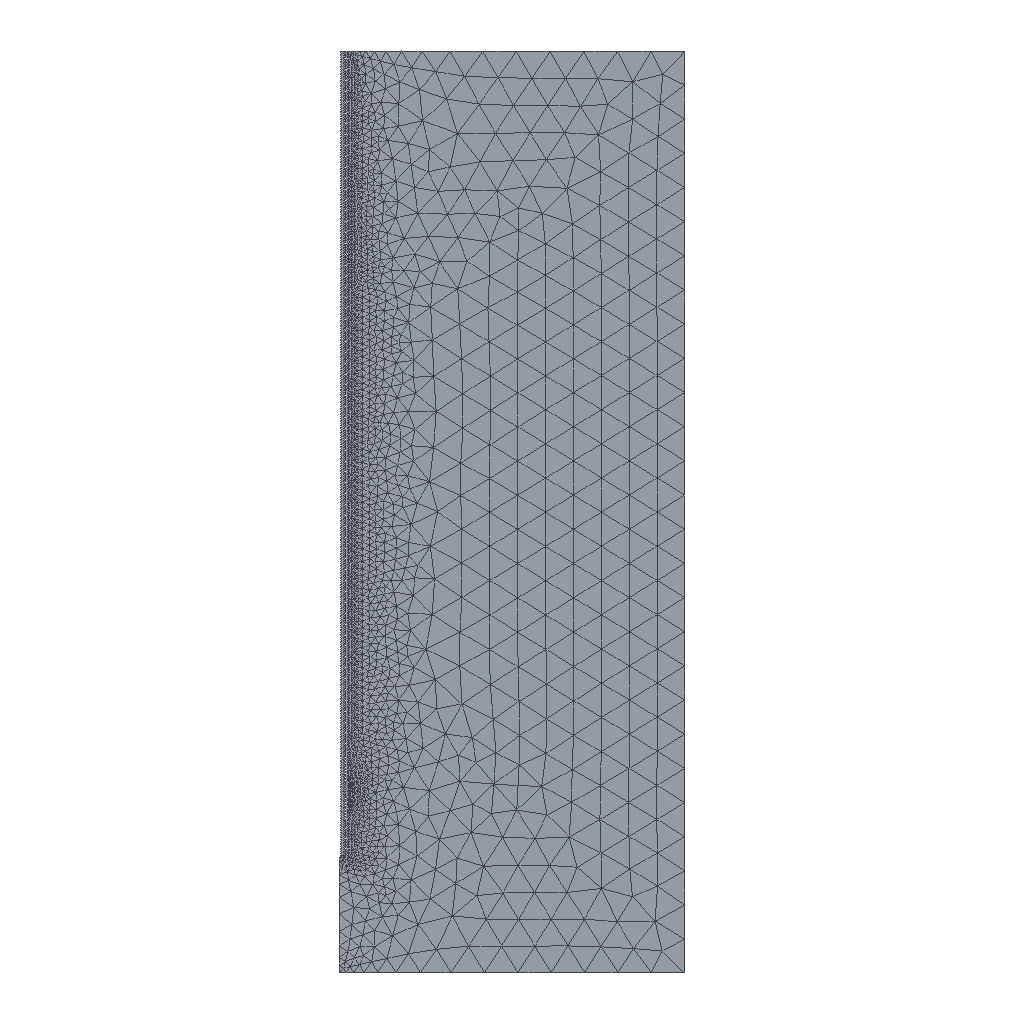Simulation study | comsol
Notes in the study folder:
k_liver 0.56[W/(m*K)] Thermal conductivity liver
rho_blood 1e3[kg/m^3] Density blood
Cp_blood 3639[J/(kg*K)] Heat capacity blood
omega_blood 3.6e-3[1/s] Blood perfusion rate
T_blood 37[degC] Temperature blood
P_in 10[W] Microwave power input
f 2.45[GHz] Microwave frequency
eps_diel 2.6[1] Dielectric relative permittivity
eps_cat 2.6[1] Catheter relative permittivity
eps_liver 43.03[1] Liver relative permittivity
sigma_liver 1.69[S/m] Conductivity liver
rho_liver 1038[kg/m^3] Liver density
Cp_liver 4187[J/(kg*K)] Liver heat capacity
sigma_cat 1e-6[S/m] Catheter conductivity
mur_cat 1[1] Catheter relative permeability
k_ptfe 0.25[W/(m*K)] Thermal conductivity PTFE
rho_ptfe 2200[kg/m^3] Density PTFE
Cp_ptfe 1300[J/(kg*K)] PTFE heat capacity
sigma_diel 1e-6[S/m] Microwave center feed
mur_diel 1[1] Relative permeability dielectric
mur_liver 1[1] Relative permeability liver
Set-up summary:
category,name,step,type,value,unit,region
solver,comsol,,COMSOL Multiphysics 6.4 (Build: 293)
units,SI; geometry length unit m,,stated,COMSOL default unit system (SI)
analysis,Study 1,,Frequency + Stationary,space_dimension=2D
load_step,std1/freq,std1/freq,Frequency + Stationary,type=Frequency; frequencies=f
load_step,std1/stat,std1/stat,Frequency + Stationary,type=Stationary
mesh,nodes,,,4184
mesh,elements,,,7113
element_type,tri,,,7113
element_type,edg,,,1524
element_type,vtx,,,18
component,mod1,,2D,geometry=geom1; domains=4
physics,Electromagnetic Waves (emw),mod1,ElectromagneticWaves,E(Er Ephi Ez)
physics,Heat Transfer (ht),mod1,BioHeat,"T(T), discontinuousdamagedtissueindicator(discontinuousdamagedtissueindicator), continuousdamagedtissueindicator(continuousdamagedtissueindicator), thermaldamageindicator(thermaldamageindicator), radiativeintensity(radiativeintensity), incidentradiation(incidentradiation), surfaceradiosity(surfaceradiosity)"
parameter,k_liver,,,0.56[W/(m*K)]
parameter,rho_blood,,,1e3[kg/m^3]
parameter,Cp_blood,,,3639[J/(kg*K)]
parameter,omega_blood,,,3.6e-3[1/s]
parameter,T_blood,,,37[degC]
parameter,P_in,,,10[W]
parameter,f,,,2.45[GHz]
parameter,eps_diel,,,2.6[1]
parameter,eps_cat,,,2.6[1]
parameter,eps_liver,,,43.03[1]
parameter,sigma_liver,,,1.69[S/m]
parameter,rho_liver,,,1038[kg/m^3]
parameter,Cp_liver,,,4187[J/(kg*K)]
parameter,sigma_cat,,,1e-6[S/m]
parameter,mur_cat,,,1[1]
parameter,k_ptfe,,,0.25[W/(m*K)]
parameter,rho_ptfe,,,2200[kg/m^3]
parameter,Cp_ptfe,,,1300[J/(kg*K)]
parameter,sigma_diel,,,1e-6[S/m]
parameter,mur_diel,,,1[1]
parameter,mur_liver,,,1[1]
material,Liver Tissue,,electricconductivity,sigma_liver,,selection [1]
material,Liver Tissue,,relpermittivity,eps_liver,,selection [1]
material,Liver Tissue,,relpermeability,mur_liver,,selection [1]
material,Liver Tissue,,thermalconductivity,k_liver,,selection [1]
material,Liver Tissue,,density,rho_liver,,selection [1]
material,Liver Tissue,,heatcapacity,Cp_liver,,selection [1]
material,Catheter,,electricconductivity,sigma_cat,,selection [2]
material,Catheter,,relpermittivity,eps_cat,,selection [2]
material,Catheter,,relpermeability,mur_cat,,selection [2]
material,Catheter,,thermalconductivity,k_ptfe,,selection [2]
material,Catheter,,density,rho_ptfe,,selection [2]
material,Catheter,,heatcapacity,Cp_ptfe,,selection [2]
material,Dielectric,,electricconductivity,sigma_diel,,selection [3]
material,Dielectric,,relpermittivity,eps_diel,,selection [3]
material,Dielectric,,relpermeability,mur_diel,,selection [3]
material,Dielectric,,thermalconductivity,k_ptfe,,selection [3]
material,Dielectric,,density,rho_ptfe,,selection [3]
material,Dielectric,,heatcapacity,Cp_ptfe,,selection [3]
material,Air,,relpermeability,1,,selection [4]
material,Air,,relpermittivity,1,,selection [4]
material,Air,,dynamicviscosity,eta(T[1/K])[Pa*s],,selection [4]
material,Air,,ratioofspecificheat,1.4,,selection [4]
material,Air,,electricconductivity,0[S/m],,selection [4]
material,Air,,heatcapacity,Cp(T[1/K])[J/(kg*K)],,selection [4]
material,Air,,density,"rho(pA[1/Pa],T[1/K])[kg/m^3]",,selection [4]
material,Air,,thermalconductivity,k(T[1/K])[W/(m*K)],,selection [4]
material,Air,,soundspeed,cs(T[1/K])[m/s],,selection [4]
bc,"Wave Equation, Electric 1 (wee1)",mod1/emw,WaveEquationElectric,,,"selection [1, 2, 3, 4]"
bc,Axial Symmetry 1 (axi1),mod1/emw,AxialSymmetry,,,"selection [1, 3]"
bc,Perfect Electric Conductor 1 (pec1),mod1/emw,PerfectElectricConductor,,,"selection [2, 5, 6, 7, 9, 11, 12, 13, 15, 17]"
bc,Initial Values 1 (init1),mod1/emw,init,,,"selection [1, 2, 3, 4]"
bc,Continuity (dcont1),mod1/emw,Continuity,,,selection []
bc,Port 1 (port1),mod1/emw,Port,,,selection [8]
bc,Scattering Boundary Condition 1 (sctr1),mod1/emw,Scattering,,,"selection [14, 18, 20, 21]"
bc,Biological Tissue 1 (bt1),mod1/ht,BiologicalTissue,,,selection [1]
bc,Axial Symmetry 1 (axi1),mod1/ht,AxialSymmetry,,,selection [1]
bc,Thermal Insulation 1 (ins1),mod1/ht,ThermalInsulation,,,"selection [2, 4, 14, 19, 20, 21]"
bc,Initial Values 1 (init1),mod1/ht,init,,,selection [1]
bc,Continuity (dcont1),mod1/ht,Continuity,,,selection []
bc,Heat Source 1 (hs1),mod1/ht,HeatSource,,,selection [1]
bc,Local Thermal Nonequilibrium Boundary 1 (ltneb1),mod1/ht,LocalThermalNonequilibriumBoundary,,,selection []
COMSOL model file for Java, long lists of numbers shortened:
/*
 * em_deck.java
 */

import com.comsol.model.*;
import com.comsol.model.util.*;

/** Model exported on Oct 28 2026, 09:08 by COMSOL 6.4.0.293. */
public class em_deck {

  public static Model run() {
    Model model = ModelUtil.create("Model");

    model.modelPath("");

    model.modelNode().create("mod1");

    model.geom().create("geom1", 2);
    model.geom("geom1").axisymmetric(true);

    model.mesh().create("mesh1", "geom1");

    model.physics().create("emw", "ElectromagneticWaves", "geom1");
    model.physics()
         .create("ht", "BioHeat", "geom1", new String[]{"I1", "I2", "I3", "I4", "I5", "I6", "I7", "I8", "I9", "I10",
         "I11", "I12"});

    model.study().create("std1");
    model.study("std1").feature().create("freq", "Frequency");

    model.name(".mph");

    model.param().set("k_liver", "0.56[W/(m*K)]");
    model.param().descr("k_liver", "Thermal conductivity liver");
    model.param().set("rho_blood", "1e3[kg/m^3]");
    model.param().descr("rho_blood", "Density blood");
    model.param().set("Cp_blood", "3639[J/(kg*K)]");
    model.param().descr("Cp_blood", "Heat capacity blood");
    model.param().set("omega_blood", "3.6e-3[1/s]");
    model.param().descr("omega_blood", "Blood perfusion rate");
    model.param().set("T_blood", "37[degC]");
    model.param().descr("T_blood", "Temperature blood");
    model.param().set("P_in", "10[W]");
    model.param().descr("P_in", "Microwave power input");
    model.param().set("f", "2.45[GHz]");
    model.param().descr("f", "Microwave frequency");
    model.param().set("eps_diel", "2.03");
    model.param().descr("eps_diel", "Dielectric relative permittivity");
    model.param().set("eps_cat", "2.6");
    model.param().descr("eps_cat", "Catheter relative permittivity");
    model.param().set("eps_liver", "43.03");
    model.param().descr("eps_liver", "Liver relative permittivity");
    model.param().set("sigma_liver", "1.69[S/m]");
    model.param().descr("sigma_liver", "Conductivity liver");
    model.param().set("rho_liver", "1038[kg/m^3]");
    model.param().descr("rho_liver", "Liver density");
    model.param().set("Cp_liver", "4187[J/(kg*K)]");
    model.param().descr("Cp_liver", "Liver heat capacity");
    model.param().set("sigma_cat", "1e-6[S/m]");
    model.param().descr("sigma_cat", "Catheter conductivity");
    model.param().set("mur_cat", "1[1]");
    model.param().descr("mur_cat", "Catheter relative permeability");
    model.param().set("k_ptfe", "0.25[W/(m*K)]");
    model.param().descr("k_ptfe", "Thermal conductivity PTFE");
    model.param().set("rho_ptfe", "2200[kg/m^3]");
    model.param().descr("rho_ptfe", "Density PTFE");
    model.param().set("Cp_ptfe", "1300[J/(kg*K)]");
    model.param().descr("Cp_ptfe", "PTFE heat capacity");
    model.param().set("sigma_diel", "1e-6[S/m]");
    model.param().descr("sigma_diel", "Microwave center feed");
    model.param().set("mur_diel", "1");
    model.param().descr("mur_diel", "Relative permeability dielectric");
    model.param().set("eps_diel", "2.03[1]");
    model.param().set("eps_cat", "2.6[1]");
    model.param().set("eps_liver", "43.03[1]");
    model.param().set("mur_diel", "1[1]");

    model.geom("geom1").feature().create("r1", "Rectangle");
    model.geom("geom1").feature("r1").setIndex("size", "0.595e-3[m]", 0);
    model.geom("geom1").feature("r1").setIndex("size", "0.01[m]", 1);
    model.geom("geom1").run("r1");
    model.geom("geom1").run("r1");
    model.geom("geom1").feature().create("r2", "Rectangle");
    model.geom("geom1").feature("r2").setIndex("size", "29.405e-3[m]", 0);
    model.geom("geom1").feature("r2").setIndex("size", "0.08[m]", 1);
    model.geom("geom1").feature("r2").setIndex("pos", "0.595e-3", 0);
    model.geom("geom1").run("r2");
    model.geom("geom1").run("r2");
    model.geom("geom1").feature().create("uni1", "Union");
    model.geom("geom1").feature("uni1").selection("input").set(new String[]{"r1", "r2"});
    model.geom("geom1").feature("uni1").set("intbnd", "off");
    model.geom("geom1").run("uni1");

    model.name(".mph");

    model.geom("geom1").run("uni1");
    model.geom("geom1").feature().create("r3", "Rectangle");
    model.geom("geom1").feature("r3").setIndex("size", "0.125e-3[m]", 0);
    model.geom("geom1").feature("r3").setIndex("size", "1.0e-3[m]", 1);
    model.geom("geom1").feature("r3").setIndex("pos", "0.47e-3[m]", 0);
    model.geom("geom1").feature("r3").setIndex("pos", "0.0155[m]", 1);
    model.geom("geom1").run("r3");
    model.geom("geom1").run("r3");
    model.geom("geom1").feature().create("r4", "Rectangle");
    model.geom("geom1").feature("r4").setIndex("size", "0.335e-3[m]", 0);
    model.geom("geom1").feature("r4").setIndex("size", "0.0699", 1);
    model.geom("geom1").feature("r4").setIndex("pos", "0.135e-3[m]", 0);
    model.geom("geom1").feature("r4").setIndex("pos", "0.0101", 1);
    model.geom("geom1").run("r4");

    model.name(".mph");

    model.geom("geom1").run("r4");
    model.geom("geom1").feature().create("b1", "BezierPolygon");
    model.geom("geom1").feature("b1").set("degree", new int[]{1});
    model.geom("geom1").feature("b1").set("p", new String[][]{{"0", "0"}, {"0", "0"}});
    model.geom("geom1").feature("b1").set("w", new String[]{"1", "1"});
    model.geom("geom1").feature("b1").setIndex("p", "0.03", 0, 1);
    model.geom("geom1").feature("b1").set("degree", new int[]{1, 1});
    model.geom("geom1").feature("b1").set("p", new String[][]{{"0", "0.03", "0.03"}, {"0", "0", "0"}});
    model.geom("geom1").feature("b1").set("w", new String[]{"1", "1", "1", "1"});
    model.geom("geom1").feature("b1").setIndex("p", "0.08", 1, 2);
    model.geom("geom1").feature("b1").set("degree", new int[]{1, 1, 1});
    model.geom("geom1").feature("b1")
         .set("p", new String[][]{{"0", "0.03", "0.03", "0.03"}, {"0", "0", "0.08", "0.08"}});
    model.geom("geom1").feature("b1").set("w", new String[]{"1", "1", "1", "1", "1", "1"});
    model.geom("geom1").feature("b1").setIndex("p", "0.0008", 0, 3);
    model.geom("geom1").feature("b1").set("degree", new int[]{1, 1, 1, 1});
    model.geom("geom1").feature("b1")
         .set("p", new String[][]{{"0", "0.03", "0.03", "0.0008", "0.0008"}, {"0", "0", "0.08", "0.08", "0.08"}});
    model.geom("geom1").feature("b1").set("w", new String[]{"1", "1", "1", "1", "1", "1", "1", "1"});
    model.geom("geom1").feature("b1").setIndex("p", "0.0098", 1, 4);
    model.geom("geom1").feature("b1").set("degree", new int[]{1, 1, 1, 1, 1});
    model.geom("geom1").feature("b1")
         .set("p", new String[][]{{"0", "0.03", "0.03", "0.0008", "0.0008", "0.0008"},
         {"0", "0", "0.08", "0.08", "0.0098", "0.0098"}});
    model.geom("geom1").feature("b1").set("w", new String[]{"1", "1", "1", "1", "1", "1", "1", "1", "1", "1"});
    model.geom("geom1").feature("b1").setIndex("p", "0.", 0, 5);
    model.geom("geom1").feature("b1").setIndex("p", "0.0092", 1, 5);
    model.geom("geom1").feature("b1").set("degree", new int[]{1, 1, 1, 1, 1, 1});
    model.geom("geom1").feature("b1")
         .set("p", new String[][]{{"0", "0.03", "0.03", "0.0008", "0.0008", "0.", "0."},
         {"0", "0", "0.08", "0.08", "0.0098", "0.0092", "0.0092"}});
    model.geom("geom1").feature("b1")
         .set("w", new String[]{"1", "1", "1", "1", "1", "1", "1", "1", "1", "1",
         "1", "1"});
    model.geom("geom1").feature("b1").setIndex("p", "0", 1, 6);
    model.geom("geom1").feature("b1")
         .set("p", new String[][]{{"0", "0.03", "0.03", "0.0008", "0.0008", "0.", "0"},
         {"0", "0", "0.08", "0.08", "0.0098", "0.0092", "0"}});
    model.geom("geom1").runAll();
    model.geom("geom1").run("b1");
    model.geom("geom1").feature().create("uni2", "Union");
    model.geom("geom1").feature("uni2").selection("input").set(new String[]{"b1", "uni1"});
    model.geom("geom1").run("uni2");

    model.name(".mph");

    model.geom("geom1").run();

    model.material().create("mat1");
    model.material("mat1").name("Liver Tissue");
    model.material("mat1").selection().set(new int[]{1});
    model.material("mat1").propertyGroup("def").set("electricconductivity", new String[]{"sigma_liver"});
    model.material("mat1").propertyGroup("def").set("relpermittivity", new String[]{"eps_liver"});

    model.param().set("mur_liver", "1[1]");
    model.param().descr("mur_liver", "Relative permeability liver");

    model.material("mat1").propertyGroup("def").set("relpermeability", new String[]{"mur_liver"});
    model.material("mat1").propertyGroup("def").set("thermalconductivity", new String[]{"k_liver"});
    model.material("mat1").propertyGroup("def").set("density", new String[]{"rho_liver"});
    model.material("mat1").propertyGroup("def").set("heatcapacity", new String[]{"Cp_liver"});
    model.material().create("mat2");
    model.material("mat2").name("Catheter");
    model.material("mat2").selection().set(new int[]{2});
    model.material("mat2").propertyGroup("def").set("electricconductivity", new String[]{"sigma_cat"});
    model.material("mat2").propertyGroup("def").set("relpermittivity", new String[]{"eps_cat"});
    model.material("mat2").propertyGroup("def").set("relpermeability", new String[]{"mur_cat"});
    model.material("mat2").propertyGroup("def").set("thermalconductivity", new String[]{"k_ptfe"});
    model.material("mat2").propertyGroup("def").set("density", new String[]{"rho_ptfe"});
    model.material("mat2").propertyGroup("def").set("heatcapacity", new String[]{"Cp_ptfe"});
    model.material().create("mat3");
    model.material("mat3").name("Dielectric");
    model.material("mat3").selection().set(new int[]{3});
    model.material("mat3").propertyGroup("def").set("electricconductivity", new String[]{"sigma_diel"});
    model.material("mat3").propertyGroup("def").set("relpermittivity", new String[]{"eps_diel"});
    model.material("mat3").propertyGroup("def").set("relpermeability", new String[]{"mur_diel"});

    model.param().set("eps_diel", "2.6[1]");

    model.material("mat3").propertyGroup("def").set("thermalconductivity", new String[]{"k_ptfe"});
    model.material("mat3").propertyGroup("def").set("density", new String[]{"rho_ptfe"});
    model.material("mat3").propertyGroup("def").set("heatcapacity", new String[]{"Cp_ptfe"});
    model.material().create("mat4");
    model.material("mat4").name("Air");
    model.material("mat4").propertyGroup("def").set("relpermeability", "1");
    model.material("mat4").propertyGroup("def").set("relpermittivity", "1");
    model.material("mat4").propertyGroup("def").set("dynamicviscosity", "eta(T[1/K])[Pa*s]");
    model.material("mat4").propertyGroup("def").set("ratioofspecificheat", "1.4");
    model.material("mat4").propertyGroup("def").set("electricconductivity", "0[S/m]");
    model.material("mat4").propertyGroup("def").set("heatcapacity", "Cp(T[1/K])[J/(kg*K)]");
    model.material("mat4").propertyGroup("def").set("density", "rho(pA[1/Pa],T[1/K])[kg/m^3]");
    model.material("mat4").propertyGroup("def").set("thermalconductivity", "k(T[1/K])[W/(m*K)]");
    model.material("mat4").propertyGroup("def").set("soundspeed", "cs(T[1/K])[m/s]");
    model.material("mat4").propertyGroup("def").func().create("eta", "Piecewise");
    model.material("mat4").propertyGroup("def").func("eta").set("funcname", "eta");
    model.material("mat4").propertyGroup("def").func("eta").set("arg", "T");
    model.material("mat4").propertyGroup("def").func("eta").set("extrap", "constant");
    model.material("mat4").propertyGroup("def").func("eta")
         .set("pieces", new String[][]{{"200.0", "1600.0", "-8.38278E-7+8.35717342E-8*T^1-7.69429583E-11*T^2+4.6437266E-14*T^3-1.06585607E-17*T^4"}});
    model.material("mat4").propertyGroup("def").func().create("Cp", "Piecewise");
    model.material("mat4").propertyGroup("def").func("Cp").set("funcname", "Cp");
    model.material("mat4").propertyGroup("def").func("Cp").set("arg", "T");
    model.material("mat4").propertyGroup("def").func("Cp").set("extrap", "constant");
    model.material("mat4").propertyGroup("def").func("Cp")
         .set("pieces", new String[][]{{"200.0", "1600.0", "1047.637-0.3726*T^1+9.45304214E-4*T^2-6.02409443E-7*T^3+1.2858961E-10*T^4"}});
    model.material("mat4").propertyGroup("def").func().create("rho", "Analytic");
    model.material("mat4").propertyGroup("def").func("rho").set("funcname", "rho");
    model.material("mat4").propertyGroup("def").func("rho").set("args", new String[]{"pA", "T"});
    model.material("mat4").propertyGroup("def").func("rho").set("expr", "pA*0.02897/8.314/T");
    model.material("mat4").propertyGroup("def").func("rho").set("dermethod", "manual");
    model.material("mat4").propertyGroup("def").func("rho")
         .set("argders", new String[][]{{"pA", "d(pA*0.02897/8.314/T,pA)"}, {"T", "d(pA*0.02897/8.314/T,T)"}});
    model.material("mat4").propertyGroup("def").func().create("k", "Piecewise");
    model.material("mat4").propertyGroup("def").func("k").set("funcname", "k");
    model.material("mat4").propertyGroup("def").func("k").set("arg", "T");
    model.material("mat4").propertyGroup("def").func("k").set("extrap", "constant");
    model.material("mat4").propertyGroup("def").func("k")
         .set("pieces", new String[][]{{"200.0", "1600.0", "-0.002276+1.15480022E-4*T^1-7.90252856E-8*T^2+4.11702505E-11*T^3-7.43864331E-15*T^4"}});
    model.material("mat4").propertyGroup("def").func().create("cs", "Analytic");
    model.material("mat4").propertyGroup("def").func("cs").set("funcname", "cs");
    model.material("mat4").propertyGroup("def").func("cs").set("args", new String[]{"T"});
    model.material("mat4").propertyGroup("def").func("cs").set("expr", "sqrt(1.4*287*T)");
    model.material("mat4").propertyGroup("def").func("cs").set("dermethod", "manual");
    model.material("mat4").propertyGroup("def").func("cs")
         .set("argders", new String[][]{{"T", "d(sqrt(1.4*287*T),T)"}});
    model.material("mat4").propertyGroup("def").addInput("temperature");
    model.material("mat4").propertyGroup("def").addInput("pressure");
    model.material("mat4").selection().set(new int[]{4});

    model.physics("emw").prop("EquationForm").set("form", 1, "Frequency");
    model.physics("emw").prop("EquationForm").set("freq_src", 1, "userdef");
    model.physics("emw").prop("EquationForm").set("freq", 1, "f");
    model.physics("emw").feature().create("port1", "Port", 1);
    model.physics("emw").feature("port1").selection().set(new int[]{8});
    model.physics("emw").feature("port1").set("PortType", 1, "Coaxial");
    model.physics("emw").feature("port1").set("PortExcitation", 1, "on");
    model.physics("emw").feature("port1").set("Pin", 1, "P_in");
    model.physics("emw").feature().create("sctr1", "Scattering", 1);
    model.physics("emw").feature("sctr1").selection().all();
    model.physics("emw").feature("sctr1").selection().set(new int[]{2, 17, 19, 20});
    model.physics("emw").feature().remove("sctr1");

    model.name(".mph");

    model.physics("emw").feature().create("sctr1", "Scattering", 1);
    model.physics("emw").feature("sctr1").selection().set(new int[]{14, 18, 20, 21});
    model.physics("ht").selection().set(new int[]{1});
    model.physics("ht").feature().create("hs1", "HeatSource", 2);
    model.physics("ht").feature("hs1").selection().all();
    model.physics("ht").feature("hs1").set("Q_src", 1, "root.mod1.emw.Qh");
    model.physics("ht").feature("bt1").feature("bh1").set("rhobl", 1, "rho_blood");
    model.physics("ht").feature("bt1").feature("bh1").set("Cb", 1, "Cp_blood");
    model.physics("ht").feature("bt1").feature("bh1").set("omegab", 1, "omega_blood");

    model.mesh("mesh1").feature().create("ftri1", "FreeTri");
    model.mesh("mesh1").feature("size").set("hmax", "3[mm]");

    model.name(".mph");

    model.mesh("mesh1").feature("ftri1").feature().create("size1", "Size");
    model.mesh("mesh1").feature("ftri1").feature("size1").selection().geom("geom1", 2);
    model.mesh("mesh1").feature("ftri1").feature("size1").selection().set(new int[]{3});
    model.mesh("mesh1").feature("ftri1").feature("size1").set("custom", "on");
    model.mesh("mesh1").feature("ftri1").feature("size1").set("hmaxactive", "on");
    model.mesh("mesh1").feature("ftri1").feature("size1").set("hmax", "0.15[mm]");
    model.mesh("mesh1").run();

    model.study("std1").feature("freq").set("plist", "f");
    model.study("std1").feature().create("stat", "Stationary");

    model.sol().create("sol1");
    model.sol("sol1").study("std1");
    model.sol("sol1").feature().create("st1", "StudyStep");
    model.sol("sol1").feature("st1").set("study", "std1");
    model.sol("sol1").feature("st1").set("studystep", "freq");
    model.sol("sol1").feature().create("v1", "Variables");
    model.sol("sol1").feature().create("s1", "Stationary");
    model.sol("sol1").feature("s1").feature().create("p1", "Parametric");
    model.sol("sol1").feature("s1").feature().remove("pDef");
    model.sol("sol1").feature("s1").feature("p1").set("pname", "freq");
    model.sol("sol1").feature("s1").feature("p1").set("plist", "f");
    model.sol("sol1").feature("s1").feature("p1").set("plot", "off");
    model.sol("sol1").feature("s1").feature("p1").set("probesel", "all");
    model.sol("sol1").feature("s1").feature("p1").set("probes", new String[]{});
    model.sol("sol1").feature("s1").feature("p1").set("control", "freq");
    model.sol("sol1").feature("s1").set("control", "freq");
    model.sol("sol1").feature("s1").feature("aDef").set("complexfun", true);
    model.sol("sol1").feature("s1").feature().create("fc1", "FullyCoupled");
    model.sol("sol1").feature("s1").feature().remove("fcDef");
    model.sol("sol1").feature().create("st2", "StudyStep");
    model.sol("sol1").feature("st2").set("study", "std1");
    model.sol("sol1").feature("st2").set("studystep", "stat");
    model.sol("sol1").feature().create("v2", "Variables");
    model.sol("sol1").feature("v2").set("initmethod", "sol");
    model.sol("sol1").feature("v2").set("initsol", "sol1");
    model.sol("sol1").feature("v2").set("notsolmethod", "sol");
    model.sol("sol1").feature("v2").set("notsol", "sol1");
    model.sol("sol1").feature().create("s2", "Stationary");
    model.sol("sol1").feature("s2").feature("aDef").set("complexfun", true);
    model.sol("sol1").feature("s2").feature().create("seDef", "Segregated");
    model.sol("sol1").feature("s2").feature().create("fc1", "FullyCoupled");
    model.sol("sol1").feature("s2").feature("fc1").set("dtech", "auto");
    model.sol("sol1").feature("s2").feature("fc1").set("initstep", 0.01);
    model.sol("sol1").feature("s2").feature("fc1").set("minstep", 1.0E-6);
    model.sol("sol1").feature("s2").feature("fc1").set("maxiter", 50);
    model.sol("sol1").feature("s2").feature().create("d1", "Direct");
    model.sol("sol1").feature("s2").feature("d1").set("linsolver", "mumps");
    model.sol("sol1").feature("s2").feature("fc1").set("linsolver", "d1");
    model.sol("sol1").feature("s2").feature("fc1").set("dtech", "auto");
    model.sol("sol1").feature("s2").feature("fc1").set("initstep", 0.01);
    model.sol("sol1").feature("s2").feature("fc1").set("minstep", 1.0E-6);
    model.sol("sol1").feature("s2").feature("fc1").set("maxiter", 50);
    model.sol("sol1").feature("s2").feature().remove("fcDef");
    model.sol("sol1").feature("s2").feature().remove("seDef");
    model.sol("sol1").attach("std1");

    model.result().create("pg1", 2);
    model.result("pg1").set("data", "dset1");
    model.result("pg1").feature().create("surf1", "Surface");
    model.result("pg1").feature("surf1").set("expr", "emw.normE");
    model.result("pg1").feature("surf1").set("descr", "Electric field norm");

    model.sol("sol1").runAll();

    model.result("pg1").set("windowtitle", "Graphics");
    model.result("pg1").run();
    model.result("pg1").run();
    model.result("pg1").run();
    model.result("pg1").feature("surf1").set("expr", "log10(mod1.emw.normE)");
    model.result("pg1").run();
    model.result("pg1").feature("surf1").set("expr", "T");
    model.result("pg1").feature("surf1").set("descr", "Temperature");
    model.result("pg1").feature("surf1").set("unit", "degC");
    model.result("pg1").run();
    model.result("pg1").run();

    model.label("in.mph");

    return model;
  }

  public static void main(String[] args) {
    run();
  }

}
Results summary:
result,max E = sqrt(abs(mod1.Er)^2+abs(mod1.Ephi)^2),dset1 (1 solution(s)),,198154,V/m
result,max T = abs(mod1.T),dset1 (1 solution(s)),,0,K